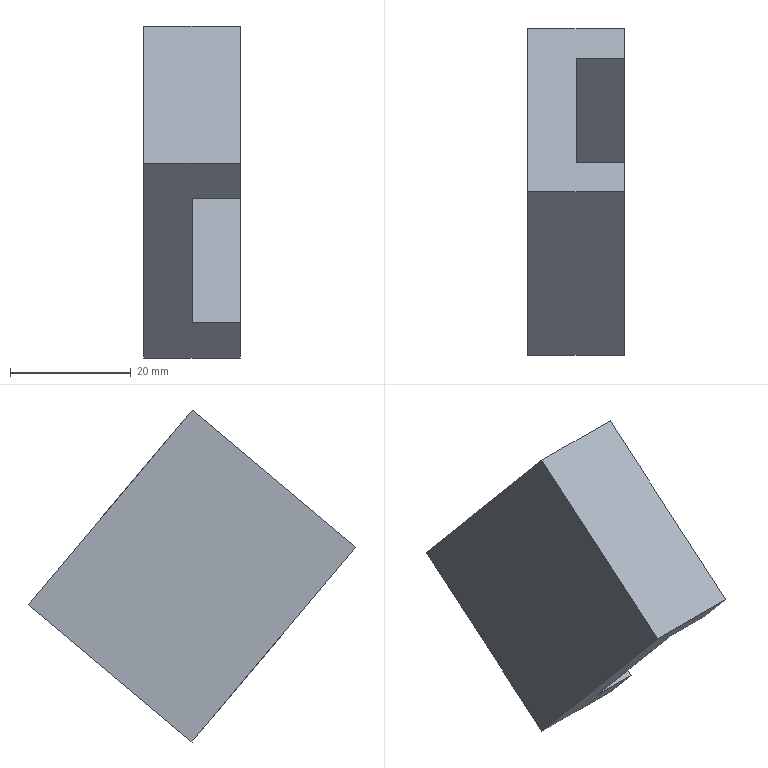Part | NX | features solid 2 | 1 solid | 10 faces | box 16 x 54.164 x 55 mm | volume 16249 mm3 | plane 10
STEP:
#1=CARTESIAN_POINT('',(-580.,766.324,84.132));
#2=VERTEX_POINT('',#1);
#3=CARTESIAN_POINT('',(-580.,783.558,63.593));
#4=VERTEX_POINT('',#3);
#5=CARTESIAN_POINT('',(-580.,761.4,90.));
#6=DIRECTION('',(0.,0.6428,-0.766));
#7=VECTOR('',#6,1000.);
#8=LINE('',#5,#7);
#9=EDGE_CURVE('',#2,#4,#8,.T.);
#10=ORIENTED_EDGE('',*,*,#9,.F.);
#11=CARTESIAN_POINT('',(-580.,739.242,61.407));
#12=VERTEX_POINT('',#11);
#13=CARTESIAN_POINT('',(-580.,761.4,80.));
#14=DIRECTION('',(0.,-0.766,-0.6428));
#15=VECTOR('',#14,1000.);
#16=LINE('',#13,#15);
#17=EDGE_CURVE('',#2,#12,#16,.T.);
#18=ORIENTED_EDGE('',*,*,#17,.T.);
#19=CARTESIAN_POINT('',(-580.,756.476,40.868));
#20=VERTEX_POINT('',#19);
#21=CARTESIAN_POINT('',(-580.,761.4,35.));
#22=DIRECTION('',(0.,-0.6428,0.766));
#23=VECTOR('',#22,1000.);
#24=LINE('',#21,#23);
#25=EDGE_CURVE('',#20,#12,#24,.T.);
#26=ORIENTED_EDGE('',*,*,#25,.F.);
#27=CARTESIAN_POINT('',(-580.,761.4,45.));
#28=DIRECTION('',(0.,-0.766,-0.6428));
#29=VECTOR('',#28,1000.);
#30=LINE('',#27,#29);
#31=EDGE_CURVE('',#4,#20,#30,.T.);
#32=ORIENTED_EDGE('',*,*,#31,.F.);
#33=EDGE_LOOP('',(#10,#18,#26,#32));
#34=FACE_BOUND('',#33,.T.);
#35=CARTESIAN_POINT('',(-580.,788.482,57.725));
#36=DIRECTION('',(1.,0.,0.));
#37=DIRECTION('',(0.,-1.,0.));
#38=AXIS2_PLACEMENT_3D('',#35,#36,#37);
#39=PLANE('',#38);
#40=ADVANCED_FACE('',(#34),#39,.T.);
#41=CARTESIAN_POINT('',(-588.,761.4,35.));
#42=VERTEX_POINT('',#41);
#43=CARTESIAN_POINT('',(-572.,761.4,35.));
#44=VERTEX_POINT('',#43);
#45=CARTESIAN_POINT('',(-588.,761.4,35.));
#46=DIRECTION('',(1.,0.,0.));
#47=VECTOR('',#46,1000.);
#48=LINE('',#45,#47);
#49=EDGE_CURVE('',#42,#44,#48,.T.);
#50=ORIENTED_EDGE('',*,*,#49,.F.);
#51=CARTESIAN_POINT('',(-588.,788.482,57.725));
#52=VERTEX_POINT('',#51);
#53=CARTESIAN_POINT('',(-588.,761.4,35.));
#54=DIRECTION('',(0.,0.766,0.6428));
#55=VECTOR('',#54,1000.);
#56=LINE('',#53,#55);
#57=EDGE_CURVE('',#42,#52,#56,.T.);
#58=ORIENTED_EDGE('',*,*,#57,.T.);
#59=CARTESIAN_POINT('',(-572.,788.482,57.725));
#60=VERTEX_POINT('',#59);
#61=CARTESIAN_POINT('',(-588.,788.482,57.725));
#62=DIRECTION('',(1.,0.,0.));
#63=VECTOR('',#62,1000.);
#64=LINE('',#61,#63);
#65=EDGE_CURVE('',#52,#60,#64,.T.);
#66=ORIENTED_EDGE('',*,*,#65,.T.);
#67=CARTESIAN_POINT('',(-572.,761.4,35.));
#68=DIRECTION('',(0.,0.766,0.6428));
#69=VECTOR('',#68,1000.);
#70=LINE('',#67,#69);
#71=EDGE_CURVE('',#44,#60,#70,.T.);
#72=ORIENTED_EDGE('',*,*,#71,.F.);
#73=EDGE_LOOP('',(#50,#58,#66,#72));
#74=FACE_BOUND('',#73,.T.);
#75=CARTESIAN_POINT('',(-588.,761.4,35.));
#76=DIRECTION('',(0.,-0.6428,0.766));
#77=DIRECTION('',(0.,0.766,0.6428));
#78=AXIS2_PLACEMENT_3D('',#75,#76,#77);
#79=PLANE('',#78);
#80=ADVANCED_FACE('',(#74),#79,.F.);
#81=ORIENTED_EDGE('',*,*,#9,.T.);
#82=CARTESIAN_POINT('',(-572.,783.558,63.593));
#83=VERTEX_POINT('',#82);
#84=CARTESIAN_POINT('',(-580.,783.558,63.593));
#85=DIRECTION('',(1.,0.,0.));
#86=VECTOR('',#85,1000.);
#87=LINE('',#84,#86);
#88=EDGE_CURVE('',#4,#83,#87,.T.);
#89=ORIENTED_EDGE('',*,*,#88,.T.);
#90=CARTESIAN_POINT('',(-572.,761.4,90.));
#91=DIRECTION('',(0.,0.6428,-0.766));
#92=VECTOR('',#91,1000.);
#93=LINE('',#90,#92);
#94=EDGE_CURVE('',#83,#60,#93,.T.);
#95=ORIENTED_EDGE('',*,*,#94,.T.);
#96=ORIENTED_EDGE('',*,*,#65,.F.);
#97=CARTESIAN_POINT('',(-588.,761.4,90.));
#98=VERTEX_POINT('',#97);
#99=CARTESIAN_POINT('',(-588.,761.4,90.));
#100=DIRECTION('',(0.,0.6428,-0.766));
#101=VECTOR('',#100,1000.);
#102=LINE('',#99,#101);
#103=EDGE_CURVE('',#98,#52,#102,.T.);
#104=ORIENTED_EDGE('',*,*,#103,.F.);
#105=CARTESIAN_POINT('',(-572.,761.4,90.));
#106=VERTEX_POINT('',#105);
#107=CARTESIAN_POINT('',(-588.,761.4,90.));
#108=DIRECTION('',(1.,0.,0.));
#109=VECTOR('',#108,1000.);
#110=LINE('',#107,#109);
#111=EDGE_CURVE('',#98,#106,#110,.T.);
#112=ORIENTED_EDGE('',*,*,#111,.T.);
#113=CARTESIAN_POINT('',(-572.,766.324,84.132));
#114=VERTEX_POINT('',#113);
#115=CARTESIAN_POINT('',(-572.,761.4,90.));
#116=DIRECTION('',(0.,0.6428,-0.766));
#117=VECTOR('',#116,1000.);
#118=LINE('',#115,#117);
#119=EDGE_CURVE('',#106,#114,#118,.T.);
#120=ORIENTED_EDGE('',*,*,#119,.T.);
#121=CARTESIAN_POINT('',(-580.,766.324,84.132));
#122=DIRECTION('',(1.,0.,0.));
#123=VECTOR('',#122,1000.);
#124=LINE('',#121,#123);
#125=EDGE_CURVE('',#2,#114,#124,.T.);
#126=ORIENTED_EDGE('',*,*,#125,.F.);
#127=EDGE_LOOP('',(#81,#89,#95,#96,#104,#112,#120,#126));
#128=FACE_BOUND('',#127,.T.);
#129=CARTESIAN_POINT('',(-588.,761.4,90.));
#130=DIRECTION('',(0.,0.766,0.6428));
#131=DIRECTION('',(0.,0.6428,-0.766));
#132=AXIS2_PLACEMENT_3D('',#129,#130,#131);
#133=PLANE('',#132);
#134=ADVANCED_FACE('',(#128),#133,.T.);
#135=ORIENTED_EDGE('',*,*,#111,.F.);
#136=CARTESIAN_POINT('',(-588.,734.318,67.275));
#137=VERTEX_POINT('',#136);
#138=CARTESIAN_POINT('',(-588.,761.4,90.));
#139=DIRECTION('',(0.,-0.766,-0.6428));
#140=VECTOR('',#139,1000.);
#141=LINE('',#138,#140);
#142=EDGE_CURVE('',#98,#137,#141,.T.);
#143=ORIENTED_EDGE('',*,*,#142,.T.);
#144=CARTESIAN_POINT('',(-572.,734.318,67.275));
#145=VERTEX_POINT('',#144);
#146=CARTESIAN_POINT('',(-588.,734.318,67.275));
#147=DIRECTION('',(1.,0.,0.));
#148=VECTOR('',#147,1000.);
#149=LINE('',#146,#148);
#150=EDGE_CURVE('',#137,#145,#149,.T.);
#151=ORIENTED_EDGE('',*,*,#150,.T.);
#152=CARTESIAN_POINT('',(-572.,761.4,90.));
#153=DIRECTION('',(0.,-0.766,-0.6428));
#154=VECTOR('',#153,1000.);
#155=LINE('',#152,#154);
#156=EDGE_CURVE('',#106,#145,#155,.T.);
#157=ORIENTED_EDGE('',*,*,#156,.F.);
#158=EDGE_LOOP('',(#135,#143,#151,#157));
#159=FACE_BOUND('',#158,.T.);
#160=CARTESIAN_POINT('',(-588.,761.4,90.));
#161=DIRECTION('',(0.,0.6428,-0.766));
#162=DIRECTION('',(0.,-0.766,-0.6428));
#163=AXIS2_PLACEMENT_3D('',#160,#161,#162);
#164=PLANE('',#163);
#165=ADVANCED_FACE('',(#159),#164,.F.);
#166=ORIENTED_EDGE('',*,*,#25,.T.);
#167=CARTESIAN_POINT('',(-572.,739.242,61.407));
#168=VERTEX_POINT('',#167);
#169=CARTESIAN_POINT('',(-580.,739.242,61.407));
#170=DIRECTION('',(1.,0.,0.));
#171=VECTOR('',#170,1000.);
#172=LINE('',#169,#171);
#173=EDGE_CURVE('',#12,#168,#172,.T.);
#174=ORIENTED_EDGE('',*,*,#173,.T.);
#175=CARTESIAN_POINT('',(-572.,761.4,35.));
#176=DIRECTION('',(0.,-0.6428,0.766));
#177=VECTOR('',#176,1000.);
#178=LINE('',#175,#177);
#179=EDGE_CURVE('',#168,#145,#178,.T.);
#180=ORIENTED_EDGE('',*,*,#179,.T.);
#181=ORIENTED_EDGE('',*,*,#150,.F.);
#182=CARTESIAN_POINT('',(-588.,761.4,35.));
#183=DIRECTION('',(0.,-0.6428,0.766));
#184=VECTOR('',#183,1000.);
#185=LINE('',#182,#184);
#186=EDGE_CURVE('',#42,#137,#185,.T.);
#187=ORIENTED_EDGE('',*,*,#186,.F.);
#188=ORIENTED_EDGE('',*,*,#49,.T.);
#189=CARTESIAN_POINT('',(-572.,756.476,40.868));
#190=VERTEX_POINT('',#189);
#191=CARTESIAN_POINT('',(-572.,761.4,35.));
#192=DIRECTION('',(0.,-0.6428,0.766));
#193=VECTOR('',#192,1000.);
#194=LINE('',#191,#193);
#195=EDGE_CURVE('',#44,#190,#194,.T.);
#196=ORIENTED_EDGE('',*,*,#195,.T.);
#197=CARTESIAN_POINT('',(-580.,756.476,40.868));
#198=DIRECTION('',(1.,0.,0.));
#199=VECTOR('',#198,1000.);
#200=LINE('',#197,#199);
#201=EDGE_CURVE('',#20,#190,#200,.T.);
#202=ORIENTED_EDGE('',*,*,#201,.F.);
#203=EDGE_LOOP('',(#166,#174,#180,#181,#187,#188,#196,#202));
#204=FACE_BOUND('',#203,.T.);
#205=CARTESIAN_POINT('',(-588.,761.4,35.));
#206=DIRECTION('',(0.,-0.766,-0.6428));
#207=DIRECTION('',(0.,-0.6428,0.766));
#208=AXIS2_PLACEMENT_3D('',#205,#206,#207);
#209=PLANE('',#208);
#210=ADVANCED_FACE('',(#204),#209,.T.);
#211=ORIENTED_EDGE('',*,*,#57,.F.);
#212=ORIENTED_EDGE('',*,*,#186,.T.);
#213=ORIENTED_EDGE('',*,*,#142,.F.);
#214=ORIENTED_EDGE('',*,*,#103,.T.);
#215=EDGE_LOOP('',(#211,#212,#213,#214));
#216=FACE_BOUND('',#215,.T.);
#217=CARTESIAN_POINT('',(-588.,788.482,57.725));
#218=DIRECTION('',(1.,0.,0.));
#219=DIRECTION('',(0.,-1.,0.));
#220=AXIS2_PLACEMENT_3D('',#217,#218,#219);
#221=PLANE('',#220);
#222=ADVANCED_FACE('',(#216),#221,.F.);
#223=CARTESIAN_POINT('',(-572.,761.4,80.));
#224=DIRECTION('',(0.,-0.766,-0.6428));
#225=VECTOR('',#224,1000.);
#226=LINE('',#223,#225);
#227=EDGE_CURVE('',#114,#168,#226,.T.);
#228=ORIENTED_EDGE('',*,*,#227,.T.);
#229=ORIENTED_EDGE('',*,*,#173,.F.);
#230=ORIENTED_EDGE('',*,*,#17,.F.);
#231=ORIENTED_EDGE('',*,*,#125,.T.);
#232=EDGE_LOOP('',(#228,#229,#230,#231));
#233=FACE_BOUND('',#232,.T.);
#234=CARTESIAN_POINT('',(-580.,761.4,80.));
#235=DIRECTION('',(0.,0.6428,-0.766));
#236=DIRECTION('',(0.,-0.766,-0.6428));
#237=AXIS2_PLACEMENT_3D('',#234,#235,#236);
#238=PLANE('',#237);
#239=ADVANCED_FACE('',(#233),#238,.T.);
#240=ORIENTED_EDGE('',*,*,#156,.T.);
#241=ORIENTED_EDGE('',*,*,#179,.F.);
#242=ORIENTED_EDGE('',*,*,#227,.F.);
#243=ORIENTED_EDGE('',*,*,#119,.F.);
#244=EDGE_LOOP('',(#240,#241,#242,#243));
#245=FACE_BOUND('',#244,.T.);
#246=CARTESIAN_POINT('',(-572.,756.969,71.281));
#247=DIRECTION('',(1.,0.,0.));
#248=DIRECTION('',(0.,-1.,0.));
#249=AXIS2_PLACEMENT_3D('',#246,#247,#248);
#250=PLANE('',#249);
#251=ADVANCED_FACE('',(#245),#250,.T.);
#252=CARTESIAN_POINT('',(-572.,761.4,45.));
#253=DIRECTION('',(0.,-0.766,-0.6428));
#254=VECTOR('',#253,1000.);
#255=LINE('',#252,#254);
#256=EDGE_CURVE('',#83,#190,#255,.T.);
#257=ORIENTED_EDGE('',*,*,#256,.F.);
#258=ORIENTED_EDGE('',*,*,#88,.F.);
#259=ORIENTED_EDGE('',*,*,#31,.T.);
#260=ORIENTED_EDGE('',*,*,#201,.T.);
#261=EDGE_LOOP('',(#257,#258,#259,#260));
#262=FACE_BOUND('',#261,.T.);
#263=CARTESIAN_POINT('',(-580.,761.4,45.));
#264=DIRECTION('',(0.,0.6428,-0.766));
#265=DIRECTION('',(0.,-0.766,-0.6428));
#266=AXIS2_PLACEMENT_3D('',#263,#264,#265);
#267=PLANE('',#266);
#268=ADVANCED_FACE('',(#262),#267,.F.);
#269=ORIENTED_EDGE('',*,*,#94,.F.);
#270=ORIENTED_EDGE('',*,*,#256,.T.);
#271=ORIENTED_EDGE('',*,*,#195,.F.);
#272=ORIENTED_EDGE('',*,*,#71,.T.);
#273=EDGE_LOOP('',(#269,#270,#271,#272));
#274=FACE_BOUND('',#273,.T.);
#275=CARTESIAN_POINT('',(-572.,766.285,54.099));
#276=DIRECTION('',(-1.,0.,0.));
#277=DIRECTION('',(0.,1.,0.));
#278=AXIS2_PLACEMENT_3D('',#275,#276,#277);
#279=PLANE('',#278);
#280=ADVANCED_FACE('',(#274),#279,.F.);
#281=CLOSED_SHELL('',(#40,#80,#134,#165,#210,#222,#239,#251,#268,#280));
#282=MANIFOLD_SOLID_BREP('',#281);
#283=(LENGTH_UNIT()NAMED_UNIT(*)SI_UNIT(.MILLI.,.METRE.));
#284=UNCERTAINTY_MEASURE_WITH_UNIT(LENGTH_MEASURE(0.00001),#283,'','');
#285=(NAMED_UNIT(*)PLANE_ANGLE_UNIT()SI_UNIT($,.RADIAN.));
#286=(NAMED_UNIT(*)SI_UNIT($,.STERADIAN.)SOLID_ANGLE_UNIT());
#287=(GEOMETRIC_REPRESENTATION_CONTEXT(3)GLOBAL_UNCERTAINTY_ASSIGNED_CONTEXT((#284))GLOBAL_UNIT_ASSIGNED_CONTEXT((#283,#285,#286))REPRESENTATION_CONTEXT('',''));
#288=ADVANCED_BREP_SHAPE_REPRESENTATION('',(#282),#287);